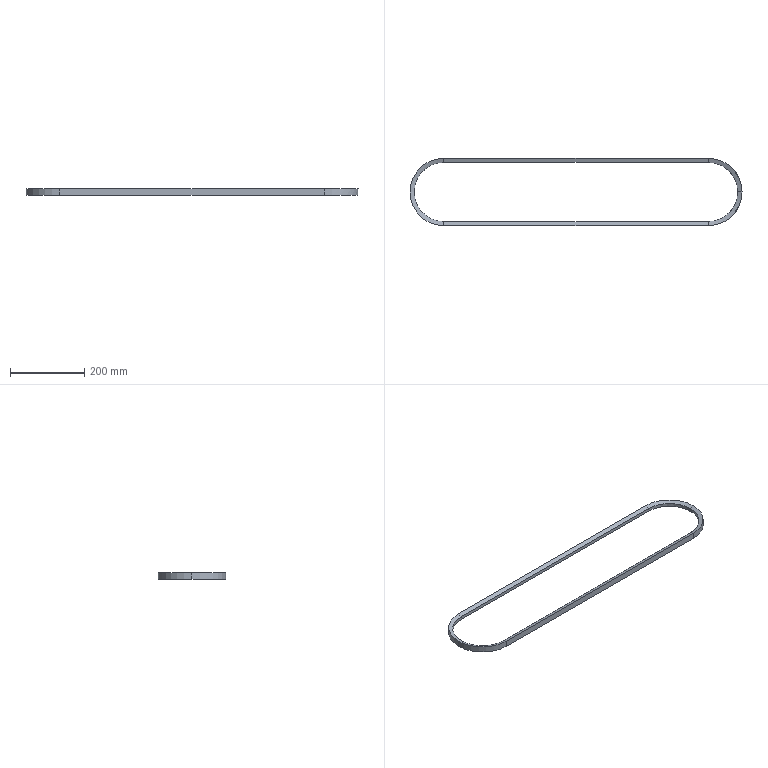Part | STEP file | Produce dryer line heating fan-BELT-B | 1 solid | 20 faces | box 896 x 182 x 17 mm | volume 281453 mm3 | plane 8 | cone 6 | cylinder 6 | commonest cylinder face diameters 160 x3 182 x3
STEP:
#1=CARTESIAN_POINT('',(714.,80.,4.496));
#2=VERTEX_POINT('',#1);
#3=CARTESIAN_POINT('',(794.,0.,4.496));
#4=VERTEX_POINT('',#3);
#5=CARTESIAN_POINT('',(714.,0.,4.496));
#6=DIRECTION('',(0.,0.,-1.));
#7=DIRECTION('',(-1.,0.,0.));
#8=AXIS2_PLACEMENT_3D('',#5,#6,#7);
#9=CIRCLE('',#8,80.);
#10=EDGE_CURVE('',#2,#4,#9,.T.);
#11=ORIENTED_EDGE('',*,*,#10,.T.);
#12=CARTESIAN_POINT('',(805.,0.,8.5));
#13=VERTEX_POINT('',#12);
#14=CARTESIAN_POINT('',(805.,0.,8.5));
#15=DIRECTION('',(0.9397,0.,0.342));
#16=VECTOR('',#15,1000.);
#17=LINE('',#14,#16);
#18=EDGE_CURVE('',#4,#13,#17,.T.);
#19=ORIENTED_EDGE('',*,*,#18,.T.);
#20=CARTESIAN_POINT('',(714.,91.,8.5));
#21=VERTEX_POINT('',#20);
#22=CARTESIAN_POINT('',(714.,0.,8.5));
#23=DIRECTION('',(0.,0.,-1.));
#24=DIRECTION('',(-1.,0.,0.));
#25=AXIS2_PLACEMENT_3D('',#22,#23,#24);
#26=CIRCLE('',#25,91.);
#27=EDGE_CURVE('',#21,#13,#26,.T.);
#28=ORIENTED_EDGE('',*,*,#27,.F.);
#29=CARTESIAN_POINT('',(714.,91.,8.5));
#30=DIRECTION('',(0.,-0.9397,-0.342));
#31=VECTOR('',#30,1000.);
#32=LINE('',#29,#31);
#33=EDGE_CURVE('',#21,#2,#32,.T.);
#34=ORIENTED_EDGE('',*,*,#33,.T.);
#35=EDGE_LOOP('',(#11,#19,#28,#34));
#36=FACE_OUTER_BOUND('',#35,.T.);
#37=CARTESIAN_POINT('',(714.,0.,8.5));
#38=DIRECTION('',(0.,0.,1.));
#39=DIRECTION('',(1.,0.,0.));
#40=AXIS2_PLACEMENT_3D('',#37,#38,#39);
#41=CONICAL_SURFACE('',#40,91.,1.222);
#42=ADVANCED_FACE('',(#36),#41,.F.);
#43=CARTESIAN_POINT('',(0.,-91.,8.5));
#44=VERTEX_POINT('',#43);
#45=CARTESIAN_POINT('',(-91.,0.,8.5));
#46=VERTEX_POINT('',#45);
#47=CARTESIAN_POINT('',(0.,0.,8.5));
#48=DIRECTION('',(0.,0.,-1.));
#49=DIRECTION('',(-1.,0.,0.));
#50=AXIS2_PLACEMENT_3D('',#47,#48,#49);
#51=CIRCLE('',#50,91.);
#52=EDGE_CURVE('',#44,#46,#51,.T.);
#53=ORIENTED_EDGE('',*,*,#52,.T.);
#54=CARTESIAN_POINT('',(-91.,0.,-8.5));
#55=VERTEX_POINT('',#54);
#56=CARTESIAN_POINT('',(-91.,0.,0.));
#57=DIRECTION('',(0.,0.,-1.));
#58=VECTOR('',#57,1000.);
#59=LINE('',#56,#58);
#60=EDGE_CURVE('',#46,#55,#59,.T.);
#61=ORIENTED_EDGE('',*,*,#60,.T.);
#62=CARTESIAN_POINT('',(0.,-91.,-8.5));
#63=VERTEX_POINT('',#62);
#64=CARTESIAN_POINT('',(0.,0.,-8.5));
#65=DIRECTION('',(0.,0.,-1.));
#66=DIRECTION('',(-1.,0.,0.));
#67=AXIS2_PLACEMENT_3D('',#64,#65,#66);
#68=CIRCLE('',#67,91.);
#69=EDGE_CURVE('',#63,#55,#68,.T.);
#70=ORIENTED_EDGE('',*,*,#69,.F.);
#71=CARTESIAN_POINT('',(0.,-91.,8.5));
#72=DIRECTION('',(0.,0.,1.));
#73=VECTOR('',#72,1000.);
#74=LINE('',#71,#73);
#75=EDGE_CURVE('',#63,#44,#74,.T.);
#76=ORIENTED_EDGE('',*,*,#75,.T.);
#77=EDGE_LOOP('',(#53,#61,#70,#76));
#78=FACE_OUTER_BOUND('',#77,.T.);
#79=CARTESIAN_POINT('',(0.,0.,0.));
#80=DIRECTION('',(0.,0.,-1.));
#81=DIRECTION('',(-1.,0.,0.));
#82=AXIS2_PLACEMENT_3D('',#79,#80,#81);
#83=CYLINDRICAL_SURFACE('',#82,91.);
#84=ADVANCED_FACE('',(#78),#83,.T.);
#85=CARTESIAN_POINT('',(-80.,0.,-4.496));
#86=VERTEX_POINT('',#85);
#87=CARTESIAN_POINT('',(0.,80.,-4.496));
#88=VERTEX_POINT('',#87);
#89=CARTESIAN_POINT('',(0.,0.,-4.496));
#90=DIRECTION('',(0.,0.,-1.));
#91=DIRECTION('',(-1.,0.,0.));
#92=AXIS2_PLACEMENT_3D('',#89,#90,#91);
#93=CIRCLE('',#92,80.);
#94=EDGE_CURVE('',#86,#88,#93,.T.);
#95=ORIENTED_EDGE('',*,*,#94,.F.);
#96=CARTESIAN_POINT('',(-80.,0.,-4.496));
#97=DIRECTION('',(-0.9397,0.,-0.342));
#98=VECTOR('',#97,1000.);
#99=LINE('',#96,#98);
#100=EDGE_CURVE('',#86,#55,#99,.T.);
#101=ORIENTED_EDGE('',*,*,#100,.T.);
#102=CARTESIAN_POINT('',(0.,91.,-8.5));
#103=VERTEX_POINT('',#102);
#104=CARTESIAN_POINT('',(0.,0.,-8.5));
#105=DIRECTION('',(0.,0.,-1.));
#106=DIRECTION('',(-1.,0.,0.));
#107=AXIS2_PLACEMENT_3D('',#104,#105,#106);
#108=CIRCLE('',#107,91.);
#109=EDGE_CURVE('',#55,#103,#108,.T.);
#110=ORIENTED_EDGE('',*,*,#109,.T.);
#111=CARTESIAN_POINT('',(0.,80.,-4.496));
#112=CARTESIAN_POINT('',(0.,83.667,-5.831));
#113=CARTESIAN_POINT('',(0.,87.333,-7.165));
#114=CARTESIAN_POINT('',(0.,91.,-8.5));
#115=B_SPLINE_CURVE_WITH_KNOTS('',3,(#111,#112,#113,#114),.UNSPECIFIED.,.F.,.F.,(4,4),(0.,1.),.UNSPECIFIED.);
#116=EDGE_CURVE('',#88,#103,#115,.T.);
#117=ORIENTED_EDGE('',*,*,#116,.F.);
#118=EDGE_LOOP('',(#95,#101,#110,#117));
#119=FACE_OUTER_BOUND('',#118,.T.);
#120=CARTESIAN_POINT('',(0.,0.,-4.496));
#121=DIRECTION('',(0.,0.,-1.));
#122=DIRECTION('',(-1.,0.,0.));
#123=AXIS2_PLACEMENT_3D('',#120,#121,#122);
#124=CONICAL_SURFACE('',#123,80.,1.222);
#125=ADVANCED_FACE('',(#119),#124,.F.);
#126=CARTESIAN_POINT('',(-80.,0.,4.496));
#127=VERTEX_POINT('',#126);
#128=CARTESIAN_POINT('',(0.,80.,4.496));
#129=VERTEX_POINT('',#128);
#130=CARTESIAN_POINT('',(0.,0.,4.496));
#131=DIRECTION('',(0.,0.,-1.));
#132=DIRECTION('',(-1.,0.,0.));
#133=AXIS2_PLACEMENT_3D('',#130,#131,#132);
#134=CIRCLE('',#133,80.);
#135=EDGE_CURVE('',#127,#129,#134,.T.);
#136=ORIENTED_EDGE('',*,*,#135,.F.);
#137=CARTESIAN_POINT('',(-80.,0.,0.));
#138=DIRECTION('',(0.,0.,-1.));
#139=VECTOR('',#138,1000.);
#140=LINE('',#137,#139);
#141=EDGE_CURVE('',#127,#86,#140,.T.);
#142=ORIENTED_EDGE('',*,*,#141,.T.);
#143=ORIENTED_EDGE('',*,*,#94,.T.);
#144=CARTESIAN_POINT('',(0.,80.,4.496));
#145=CARTESIAN_POINT('',(0.,80.,1.499));
#146=CARTESIAN_POINT('',(0.,80.,-1.499));
#147=CARTESIAN_POINT('',(0.,80.,-4.496));
#148=B_SPLINE_CURVE_WITH_KNOTS('',3,(#144,#145,#146,#147),.UNSPECIFIED.,.F.,.F.,(4,4),(0.,1.),.UNSPECIFIED.);
#149=EDGE_CURVE('',#129,#88,#148,.T.);
#150=ORIENTED_EDGE('',*,*,#149,.F.);
#151=EDGE_LOOP('',(#136,#142,#143,#150));
#152=FACE_OUTER_BOUND('',#151,.T.);
#153=CARTESIAN_POINT('',(0.,0.,0.));
#154=DIRECTION('',(0.,0.,-1.));
#155=DIRECTION('',(-1.,0.,0.));
#156=AXIS2_PLACEMENT_3D('',#153,#154,#155);
#157=CYLINDRICAL_SURFACE('',#156,80.);
#158=ADVANCED_FACE('',(#152),#157,.F.);
#159=ORIENTED_EDGE('',*,*,#141,.F.);
#160=CARTESIAN_POINT('',(0.,-80.,4.496));
#161=VERTEX_POINT('',#160);
#162=CARTESIAN_POINT('',(0.,0.,4.496));
#163=DIRECTION('',(0.,0.,-1.));
#164=DIRECTION('',(-1.,0.,0.));
#165=AXIS2_PLACEMENT_3D('',#162,#163,#164);
#166=CIRCLE('',#165,80.);
#167=EDGE_CURVE('',#161,#127,#166,.T.);
#168=ORIENTED_EDGE('',*,*,#167,.F.);
#169=CARTESIAN_POINT('',(0.,-80.,-4.496));
#170=VERTEX_POINT('',#169);
#171=CARTESIAN_POINT('',(0.,-80.,4.496));
#172=DIRECTION('',(0.,0.,-1.));
#173=VECTOR('',#172,1000.);
#174=LINE('',#171,#173);
#175=EDGE_CURVE('',#161,#170,#174,.T.);
#176=ORIENTED_EDGE('',*,*,#175,.T.);
#177=CARTESIAN_POINT('',(0.,0.,-4.496));
#178=DIRECTION('',(0.,0.,-1.));
#179=DIRECTION('',(-1.,0.,0.));
#180=AXIS2_PLACEMENT_3D('',#177,#178,#179);
#181=CIRCLE('',#180,80.);
#182=EDGE_CURVE('',#170,#86,#181,.T.);
#183=ORIENTED_EDGE('',*,*,#182,.T.);
#184=EDGE_LOOP('',(#159,#168,#176,#183));
#185=FACE_OUTER_BOUND('',#184,.T.);
#186=CARTESIAN_POINT('',(0.,0.,0.));
#187=DIRECTION('',(0.,0.,-1.));
#188=DIRECTION('',(-1.,0.,0.));
#189=AXIS2_PLACEMENT_3D('',#186,#187,#188);
#190=CYLINDRICAL_SURFACE('',#189,80.);
#191=ADVANCED_FACE('',(#185),#190,.F.);
#192=ORIENTED_EDGE('',*,*,#100,.F.);
#193=ORIENTED_EDGE('',*,*,#182,.F.);
#194=CARTESIAN_POINT('',(0.,-80.,-4.496));
#195=DIRECTION('',(0.,-0.9397,-0.342));
#196=VECTOR('',#195,1000.);
#197=LINE('',#194,#196);
#198=EDGE_CURVE('',#170,#63,#197,.T.);
#199=ORIENTED_EDGE('',*,*,#198,.T.);
#200=ORIENTED_EDGE('',*,*,#69,.T.);
#201=EDGE_LOOP('',(#192,#193,#199,#200));
#202=FACE_OUTER_BOUND('',#201,.T.);
#203=CARTESIAN_POINT('',(0.,0.,-4.496));
#204=DIRECTION('',(0.,0.,-1.));
#205=DIRECTION('',(-1.,0.,0.));
#206=AXIS2_PLACEMENT_3D('',#203,#204,#205);
#207=CONICAL_SURFACE('',#206,80.,1.222);
#208=ADVANCED_FACE('',(#202),#207,.F.);
#209=ORIENTED_EDGE('',*,*,#60,.F.);
#210=CARTESIAN_POINT('',(0.,91.,8.5));
#211=VERTEX_POINT('',#210);
#212=CARTESIAN_POINT('',(0.,0.,8.5));
#213=DIRECTION('',(0.,0.,-1.));
#214=DIRECTION('',(-1.,0.,0.));
#215=AXIS2_PLACEMENT_3D('',#212,#213,#214);
#216=CIRCLE('',#215,91.);
#217=EDGE_CURVE('',#46,#211,#216,.T.);
#218=ORIENTED_EDGE('',*,*,#217,.T.);
#219=CARTESIAN_POINT('',(0.,91.,-8.5));
#220=CARTESIAN_POINT('',(0.,91.,-2.833));
#221=CARTESIAN_POINT('',(0.,91.,2.833));
#222=CARTESIAN_POINT('',(0.,91.,8.5));
#223=B_SPLINE_CURVE_WITH_KNOTS('',3,(#219,#220,#221,#222),.UNSPECIFIED.,.F.,.F.,(4,4),(0.,1.),.UNSPECIFIED.);
#224=EDGE_CURVE('',#103,#211,#223,.T.);
#225=ORIENTED_EDGE('',*,*,#224,.F.);
#226=ORIENTED_EDGE('',*,*,#109,.F.);
#227=EDGE_LOOP('',(#209,#218,#225,#226));
#228=FACE_OUTER_BOUND('',#227,.T.);
#229=CARTESIAN_POINT('',(0.,0.,0.));
#230=DIRECTION('',(0.,0.,-1.));
#231=DIRECTION('',(-1.,0.,0.));
#232=AXIS2_PLACEMENT_3D('',#229,#230,#231);
#233=CYLINDRICAL_SURFACE('',#232,91.);
#234=ADVANCED_FACE('',(#228),#233,.T.);
#235=CARTESIAN_POINT('',(0.,-91.,8.5));
#236=DIRECTION('',(0.,0.9397,-0.342));
#237=VECTOR('',#236,1000.);
#238=LINE('',#235,#237);
#239=EDGE_CURVE('',#44,#161,#238,.T.);
#240=ORIENTED_EDGE('',*,*,#239,.T.);
#241=ORIENTED_EDGE('',*,*,#167,.T.);
#242=ORIENTED_EDGE('',*,*,#135,.T.);
#243=CARTESIAN_POINT('',(0.,91.,8.5));
#244=CARTESIAN_POINT('',(0.,87.333,7.165));
#245=CARTESIAN_POINT('',(0.,83.667,5.831));
#246=CARTESIAN_POINT('',(0.,80.,4.496));
#247=B_SPLINE_CURVE_WITH_KNOTS('',3,(#243,#244,#245,#246),.UNSPECIFIED.,.F.,.F.,(4,4),(0.,1.),.UNSPECIFIED.);
#248=EDGE_CURVE('',#211,#129,#247,.T.);
#249=ORIENTED_EDGE('',*,*,#248,.F.);
#250=ORIENTED_EDGE('',*,*,#217,.F.);
#251=ORIENTED_EDGE('',*,*,#52,.F.);
#252=EDGE_LOOP('',(#240,#241,#242,#249,#250,#251));
#253=FACE_OUTER_BOUND('',#252,.T.);
#254=CARTESIAN_POINT('',(0.,0.,8.5));
#255=DIRECTION('',(0.,0.,1.));
#256=DIRECTION('',(1.,0.,0.));
#257=AXIS2_PLACEMENT_3D('',#254,#255,#256);
#258=CONICAL_SURFACE('',#257,91.,1.222);
#259=ADVANCED_FACE('',(#253),#258,.F.);
#260=CARTESIAN_POINT('',(714.,-80.,4.496));
#261=VERTEX_POINT('',#260);
#262=CARTESIAN_POINT('',(714.,-80.,-4.496));
#263=VERTEX_POINT('',#262);
#264=CARTESIAN_POINT('',(714.,-80.,4.496));
#265=DIRECTION('',(0.,0.,-1.));
#266=VECTOR('',#265,1000.);
#267=LINE('',#264,#266);
#268=EDGE_CURVE('',#261,#263,#267,.T.);
#269=ORIENTED_EDGE('',*,*,#268,.T.);
#270=CARTESIAN_POINT('',(714.,-80.,-4.496));
#271=DIRECTION('',(-1.,0.,0.));
#272=VECTOR('',#271,1000.);
#273=LINE('',#270,#272);
#274=EDGE_CURVE('',#263,#170,#273,.T.);
#275=ORIENTED_EDGE('',*,*,#274,.T.);
#276=ORIENTED_EDGE('',*,*,#175,.F.);
#277=CARTESIAN_POINT('',(714.,-80.,4.496));
#278=DIRECTION('',(-1.,0.,0.));
#279=VECTOR('',#278,1000.);
#280=LINE('',#277,#279);
#281=EDGE_CURVE('',#261,#161,#280,.T.);
#282=ORIENTED_EDGE('',*,*,#281,.F.);
#283=EDGE_LOOP('',(#269,#275,#276,#282));
#284=FACE_OUTER_BOUND('',#283,.T.);
#285=CARTESIAN_POINT('',(714.,-80.,4.496));
#286=DIRECTION('',(0.,1.,0.));
#287=DIRECTION('',(-1.,0.,0.));
#288=AXIS2_PLACEMENT_3D('',#285,#286,#287);
#289=PLANE('',#288);
#290=ADVANCED_FACE('',(#284),#289,.T.);
#291=CARTESIAN_POINT('',(714.,-91.,-8.5));
#292=VERTEX_POINT('',#291);
#293=CARTESIAN_POINT('',(714.,-80.,-4.496));
#294=DIRECTION('',(0.,-0.9397,-0.342));
#295=VECTOR('',#294,1000.);
#296=LINE('',#293,#295);
#297=EDGE_CURVE('',#263,#292,#296,.T.);
#298=ORIENTED_EDGE('',*,*,#297,.T.);
#299=CARTESIAN_POINT('',(714.,-91.,-8.5));
#300=DIRECTION('',(-1.,0.,0.));
#301=VECTOR('',#300,1000.);
#302=LINE('',#299,#301);
#303=EDGE_CURVE('',#292,#63,#302,.T.);
#304=ORIENTED_EDGE('',*,*,#303,.T.);
#305=ORIENTED_EDGE('',*,*,#198,.F.);
#306=ORIENTED_EDGE('',*,*,#274,.F.);
#307=EDGE_LOOP('',(#298,#304,#305,#306));
#308=FACE_OUTER_BOUND('',#307,.T.);
#309=CARTESIAN_POINT('',(714.,-80.,-4.496));
#310=DIRECTION('',(0.,0.342,-0.9397));
#311=DIRECTION('',(0.,0.9397,0.342));
#312=AXIS2_PLACEMENT_3D('',#309,#310,#311);
#313=PLANE('',#312);
#314=ADVANCED_FACE('',(#308),#313,.T.);
#315=CARTESIAN_POINT('',(714.,-91.,8.5));
#316=VERTEX_POINT('',#315);
#317=CARTESIAN_POINT('',(714.,-91.,8.5));
#318=DIRECTION('',(0.,0.,1.));
#319=VECTOR('',#318,1000.);
#320=LINE('',#317,#319);
#321=EDGE_CURVE('',#292,#316,#320,.T.);
#322=ORIENTED_EDGE('',*,*,#321,.T.);
#323=CARTESIAN_POINT('',(714.,-91.,8.5));
#324=DIRECTION('',(-1.,0.,0.));
#325=VECTOR('',#324,1000.);
#326=LINE('',#323,#325);
#327=EDGE_CURVE('',#316,#44,#326,.T.);
#328=ORIENTED_EDGE('',*,*,#327,.T.);
#329=ORIENTED_EDGE('',*,*,#75,.F.);
#330=ORIENTED_EDGE('',*,*,#303,.F.);
#331=EDGE_LOOP('',(#322,#328,#329,#330));
#332=FACE_OUTER_BOUND('',#331,.T.);
#333=CARTESIAN_POINT('',(714.,-91.,8.5));
#334=DIRECTION('',(0.,-1.,0.));
#335=DIRECTION('',(1.,0.,0.));
#336=AXIS2_PLACEMENT_3D('',#333,#334,#335);
#337=PLANE('',#336);
#338=ADVANCED_FACE('',(#332),#337,.T.);
#339=CARTESIAN_POINT('',(714.,-91.,8.5));
#340=DIRECTION('',(0.,0.9397,-0.342));
#341=VECTOR('',#340,1000.);
#342=LINE('',#339,#341);
#343=EDGE_CURVE('',#316,#261,#342,.T.);
#344=ORIENTED_EDGE('',*,*,#343,.T.);
#345=ORIENTED_EDGE('',*,*,#281,.T.);
#346=ORIENTED_EDGE('',*,*,#239,.F.);
#347=ORIENTED_EDGE('',*,*,#327,.F.);
#348=EDGE_LOOP('',(#344,#345,#346,#347));
#349=FACE_OUTER_BOUND('',#348,.T.);
#350=CARTESIAN_POINT('',(714.,-91.,8.5));
#351=DIRECTION('',(0.,0.342,0.9397));
#352=DIRECTION('',(0.,-0.9397,0.342));
#353=AXIS2_PLACEMENT_3D('',#350,#351,#352);
#354=PLANE('',#353);
#355=ADVANCED_FACE('',(#349),#354,.T.);
#356=CARTESIAN_POINT('',(714.,80.,-4.496));
#357=VERTEX_POINT('',#356);
#358=CARTESIAN_POINT('',(714.,80.,4.496));
#359=DIRECTION('',(0.,0.,-1.));
#360=VECTOR('',#359,1000.);
#361=LINE('',#358,#360);
#362=EDGE_CURVE('',#2,#357,#361,.T.);
#363=ORIENTED_EDGE('',*,*,#362,.T.);
#364=CARTESIAN_POINT('',(714.,0.,-4.496));
#365=DIRECTION('',(0.,0.,-1.));
#366=DIRECTION('',(-1.,0.,0.));
#367=AXIS2_PLACEMENT_3D('',#364,#365,#366);
#368=CIRCLE('',#367,80.);
#369=EDGE_CURVE('',#357,#263,#368,.T.);
#370=ORIENTED_EDGE('',*,*,#369,.T.);
#371=ORIENTED_EDGE('',*,*,#268,.F.);
#372=CARTESIAN_POINT('',(714.,0.,4.496));
#373=DIRECTION('',(0.,0.,-1.));
#374=DIRECTION('',(-1.,0.,0.));
#375=AXIS2_PLACEMENT_3D('',#372,#373,#374);
#376=CIRCLE('',#375,80.);
#377=EDGE_CURVE('',#4,#261,#376,.T.);
#378=ORIENTED_EDGE('',*,*,#377,.F.);
#379=ORIENTED_EDGE('',*,*,#10,.F.);
#380=EDGE_LOOP('',(#363,#370,#371,#378,#379));
#381=FACE_OUTER_BOUND('',#380,.T.);
#382=CARTESIAN_POINT('',(714.,0.,0.));
#383=DIRECTION('',(0.,0.,-1.));
#384=DIRECTION('',(-1.,0.,0.));
#385=AXIS2_PLACEMENT_3D('',#382,#383,#384);
#386=CYLINDRICAL_SURFACE('',#385,80.);
#387=ADVANCED_FACE('',(#381),#386,.F.);
#388=CARTESIAN_POINT('',(714.,91.,-8.5));
#389=VERTEX_POINT('',#388);
#390=CARTESIAN_POINT('',(714.,80.,-4.496));
#391=DIRECTION('',(0.,0.9397,-0.342));
#392=VECTOR('',#391,1000.);
#393=LINE('',#390,#392);
#394=EDGE_CURVE('',#357,#389,#393,.T.);
#395=ORIENTED_EDGE('',*,*,#394,.T.);
#396=CARTESIAN_POINT('',(714.,0.,-8.5));
#397=DIRECTION('',(0.,0.,-1.));
#398=DIRECTION('',(-1.,0.,0.));
#399=AXIS2_PLACEMENT_3D('',#396,#397,#398);
#400=CIRCLE('',#399,91.);
#401=EDGE_CURVE('',#389,#292,#400,.T.);
#402=ORIENTED_EDGE('',*,*,#401,.T.);
#403=ORIENTED_EDGE('',*,*,#297,.F.);
#404=ORIENTED_EDGE('',*,*,#369,.F.);
#405=EDGE_LOOP('',(#395,#402,#403,#404));
#406=FACE_OUTER_BOUND('',#405,.T.);
#407=CARTESIAN_POINT('',(714.,0.,-4.496));
#408=DIRECTION('',(0.,0.,-1.));
#409=DIRECTION('',(-1.,0.,0.));
#410=AXIS2_PLACEMENT_3D('',#407,#408,#409);
#411=CONICAL_SURFACE('',#410,80.,1.222);
#412=ADVANCED_FACE('',(#406),#411,.F.);
#413=CARTESIAN_POINT('',(714.,91.,8.5));
#414=DIRECTION('',(0.,0.,1.));
#415=VECTOR('',#414,1000.);
#416=LINE('',#413,#415);
#417=EDGE_CURVE('',#389,#21,#416,.T.);
#418=ORIENTED_EDGE('',*,*,#417,.T.);
#419=ORIENTED_EDGE('',*,*,#27,.T.);
#420=CARTESIAN_POINT('',(714.,0.,8.5));
#421=DIRECTION('',(0.,0.,-1.));
#422=DIRECTION('',(-1.,0.,0.));
#423=AXIS2_PLACEMENT_3D('',#420,#421,#422);
#424=CIRCLE('',#423,91.);
#425=EDGE_CURVE('',#13,#316,#424,.T.);
#426=ORIENTED_EDGE('',*,*,#425,.T.);
#427=ORIENTED_EDGE('',*,*,#321,.F.);
#428=ORIENTED_EDGE('',*,*,#401,.F.);
#429=EDGE_LOOP('',(#418,#419,#426,#427,#428));
#430=FACE_OUTER_BOUND('',#429,.T.);
#431=CARTESIAN_POINT('',(714.,0.,0.));
#432=DIRECTION('',(0.,0.,-1.));
#433=DIRECTION('',(-1.,0.,0.));
#434=AXIS2_PLACEMENT_3D('',#431,#432,#433);
#435=CYLINDRICAL_SURFACE('',#434,91.);
#436=ADVANCED_FACE('',(#430),#435,.T.);
#437=ORIENTED_EDGE('',*,*,#18,.F.);
#438=ORIENTED_EDGE('',*,*,#377,.T.);
#439=ORIENTED_EDGE('',*,*,#343,.F.);
#440=ORIENTED_EDGE('',*,*,#425,.F.);
#441=EDGE_LOOP('',(#437,#438,#439,#440));
#442=FACE_OUTER_BOUND('',#441,.T.);
#443=CARTESIAN_POINT('',(714.,0.,8.5));
#444=DIRECTION('',(0.,0.,1.));
#445=DIRECTION('',(1.,0.,0.));
#446=AXIS2_PLACEMENT_3D('',#443,#444,#445);
#447=CONICAL_SURFACE('',#446,91.,1.222);
#448=ADVANCED_FACE('',(#442),#447,.F.);
#449=ORIENTED_EDGE('',*,*,#248,.T.);
#450=CARTESIAN_POINT('',(714.,80.,4.496));
#451=DIRECTION('',(-1.,0.,0.));
#452=VECTOR('',#451,1000.);
#453=LINE('',#450,#452);
#454=EDGE_CURVE('',#2,#129,#453,.T.);
#455=ORIENTED_EDGE('',*,*,#454,.F.);
#456=ORIENTED_EDGE('',*,*,#33,.F.);
#457=CARTESIAN_POINT('',(714.,91.,8.5));
#458=DIRECTION('',(-1.,0.,0.));
#459=VECTOR('',#458,1000.);
#460=LINE('',#457,#459);
#461=EDGE_CURVE('',#21,#211,#460,.T.);
#462=ORIENTED_EDGE('',*,*,#461,.T.);
#463=EDGE_LOOP('',(#449,#455,#456,#462));
#464=FACE_OUTER_BOUND('',#463,.T.);
#465=CARTESIAN_POINT('',(714.,91.,8.5));
#466=DIRECTION('',(0.,0.342,-0.9397));
#467=DIRECTION('',(0.,0.9397,0.342));
#468=AXIS2_PLACEMENT_3D('',#465,#466,#467);
#469=PLANE('',#468);
#470=ADVANCED_FACE('',(#464),#469,.F.);
#471=ORIENTED_EDGE('',*,*,#149,.T.);
#472=CARTESIAN_POINT('',(714.,80.,-4.496));
#473=DIRECTION('',(-1.,0.,0.));
#474=VECTOR('',#473,1000.);
#475=LINE('',#472,#474);
#476=EDGE_CURVE('',#357,#88,#475,.T.);
#477=ORIENTED_EDGE('',*,*,#476,.F.);
#478=ORIENTED_EDGE('',*,*,#362,.F.);
#479=ORIENTED_EDGE('',*,*,#454,.T.);
#480=EDGE_LOOP('',(#471,#477,#478,#479));
#481=FACE_OUTER_BOUND('',#480,.T.);
#482=CARTESIAN_POINT('',(714.,80.,4.496));
#483=DIRECTION('',(0.,1.,0.));
#484=DIRECTION('',(-1.,0.,0.));
#485=AXIS2_PLACEMENT_3D('',#482,#483,#484);
#486=PLANE('',#485);
#487=ADVANCED_FACE('',(#481),#486,.F.);
#488=ORIENTED_EDGE('',*,*,#116,.T.);
#489=CARTESIAN_POINT('',(714.,91.,-8.5));
#490=DIRECTION('',(-1.,0.,0.));
#491=VECTOR('',#490,1000.);
#492=LINE('',#489,#491);
#493=EDGE_CURVE('',#389,#103,#492,.T.);
#494=ORIENTED_EDGE('',*,*,#493,.F.);
#495=ORIENTED_EDGE('',*,*,#394,.F.);
#496=ORIENTED_EDGE('',*,*,#476,.T.);
#497=EDGE_LOOP('',(#488,#494,#495,#496));
#498=FACE_OUTER_BOUND('',#497,.T.);
#499=CARTESIAN_POINT('',(714.,80.,-4.496));
#500=DIRECTION('',(0.,0.342,0.9397));
#501=DIRECTION('',(0.,-0.9397,0.342));
#502=AXIS2_PLACEMENT_3D('',#499,#500,#501);
#503=PLANE('',#502);
#504=ADVANCED_FACE('',(#498),#503,.F.);
#505=ORIENTED_EDGE('',*,*,#224,.T.);
#506=ORIENTED_EDGE('',*,*,#461,.F.);
#507=ORIENTED_EDGE('',*,*,#417,.F.);
#508=ORIENTED_EDGE('',*,*,#493,.T.);
#509=EDGE_LOOP('',(#505,#506,#507,#508));
#510=FACE_OUTER_BOUND('',#509,.T.);
#511=CARTESIAN_POINT('',(714.,91.,8.5));
#512=DIRECTION('',(0.,-1.,0.));
#513=DIRECTION('',(1.,0.,0.));
#514=AXIS2_PLACEMENT_3D('',#511,#512,#513);
#515=PLANE('',#514);
#516=ADVANCED_FACE('',(#510),#515,.F.);
#517=CLOSED_SHELL('',(#42,#84,#125,#158,#191,#208,#234,#259,#290,#314,#338,#355,#387,#412,#436,#448,#470,#487,#504,#516));
#518=MANIFOLD_SOLID_BREP('',#517);
#519=CARTESIAN_POINT('',(0.,0.,0.));
#520=DIRECTION('',(0.,0.,1.));
#521=DIRECTION('',(1.,0.,0.));
#522=AXIS2_PLACEMENT_3D('',#519,#520,#521);
#523=(LENGTH_UNIT()NAMED_UNIT(*)SI_UNIT(.MILLI.,.METRE.));
#524=UNCERTAINTY_MEASURE_WITH_UNIT(LENGTH_MEASURE(0.00001),#523,'','');
#525=(NAMED_UNIT(*)PLANE_ANGLE_UNIT()SI_UNIT($,.RADIAN.));
#526=(NAMED_UNIT(*)SI_UNIT($,.STERADIAN.)SOLID_ANGLE_UNIT());
#527=(GEOMETRIC_REPRESENTATION_CONTEXT(3)GLOBAL_UNCERTAINTY_ASSIGNED_CONTEXT((#524))GLOBAL_UNIT_ASSIGNED_CONTEXT((#523,#525,#526))REPRESENTATION_CONTEXT('',''));
#528=ADVANCED_BREP_SHAPE_REPRESENTATION('',(#518,#522),#527);